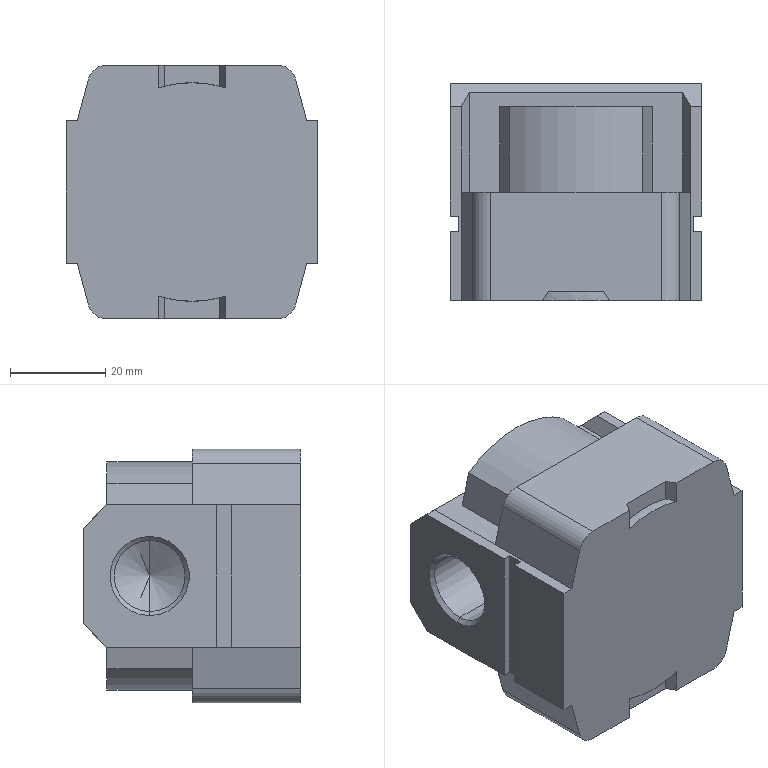Part | SolidWorks | features ICE 7, RefAxis 6, HoleWzd 3, 3DProfileFeature 2, Extrusion 1, LPattern 1, Revolution 1 | 1 solid | 97 faces | box 53 x 45.8 x 53.4 mm | volume 95835 mm3 | plane 52 | cone 24 | cylinder 21 | commonest cylinder face diameters 3.242 x8 8 x4 14.95 x4 48 x3 46 x2